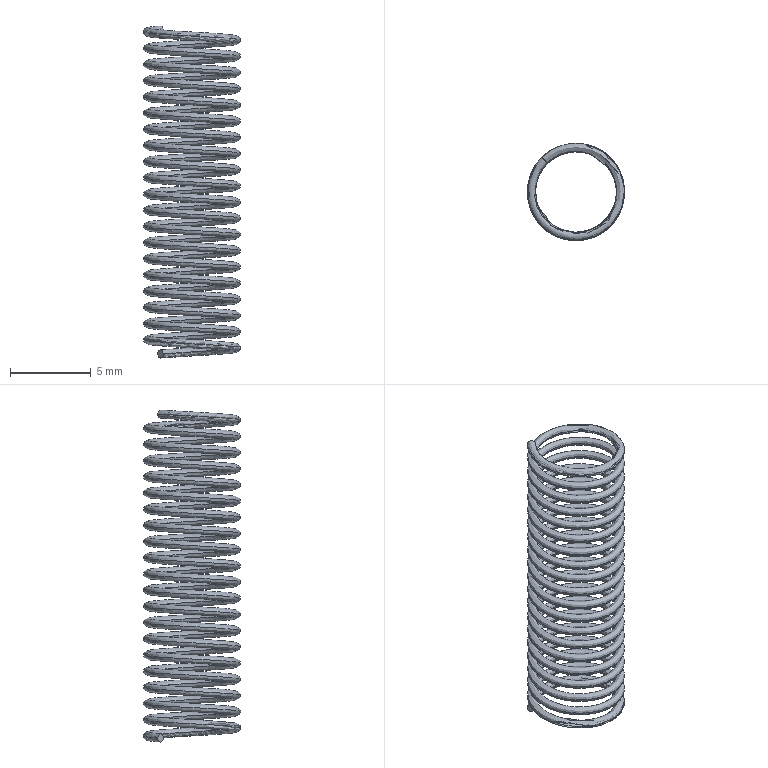Part | STEP file | spring | 1 solid | 6 faces | box 5.998 x 5.998 x 20.499 mm | volume 67.793 mm3 | plane 3 | spline 2 | cylinder 1 | commonest cylinder face diameters 5 x1